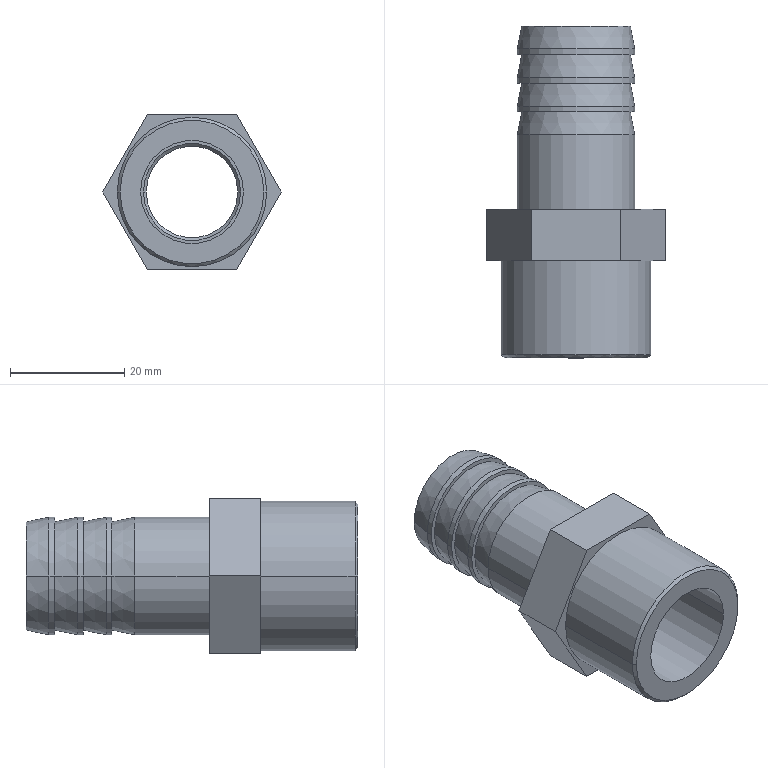Part | SolidWorks | features ICE 4, Chamfer 2, Revolution 1 | 1 solid | 40 faces | box 31.177 x 58 x 27 mm | volume 12376 mm3 | cylinder 14 | plane 14 | cone 12 | commonest cylinder face diameters 20.5 x8 16 x2 18 x2 26.1 x2
STEP:
#1=CARTESIAN_POINT('',(-8.,-8.5,0.));
#2=VERTEX_POINT('',#1);
#3=CARTESIAN_POINT('',(8.,-8.5,0.));
#4=VERTEX_POINT('',#3);
#5=CARTESIAN_POINT('',(0.,-8.5,0.));
#6=DIRECTION('',(0.,-1.,0.));
#7=DIRECTION('',(1.,0.,0.));
#8=AXIS2_PLACEMENT_3D('',#5,#6,#7);
#9=CIRCLE('',#8,8.);
#10=EDGE_CURVE('',#2,#4,#9,.T.);
#11=ORIENTED_EDGE('',*,*,#10,.F.);
#12=CARTESIAN_POINT('',(-8.5,-9.,0.));
#13=VERTEX_POINT('',#12);
#14=CARTESIAN_POINT('',(-8.5,-9.,0.));
#15=DIRECTION('',(-0.7071,-0.7071,0.));
#16=VECTOR('',#15,1000.);
#17=LINE('',#14,#16);
#18=EDGE_CURVE('',#2,#13,#17,.T.);
#19=ORIENTED_EDGE('',*,*,#18,.T.);
#20=CARTESIAN_POINT('',(8.5,-9.,0.));
#21=VERTEX_POINT('',#20);
#22=CARTESIAN_POINT('',(0.,-9.,0.));
#23=DIRECTION('',(0.,1.,0.));
#24=DIRECTION('',(1.,0.,0.));
#25=AXIS2_PLACEMENT_3D('',#22,#23,#24);
#26=CIRCLE('',#25,8.5);
#27=EDGE_CURVE('',#21,#13,#26,.T.);
#28=ORIENTED_EDGE('',*,*,#27,.F.);
#29=CARTESIAN_POINT('',(8.5,-9.,0.));
#30=DIRECTION('',(0.7071,-0.7071,0.));
#31=VECTOR('',#30,1000.);
#32=LINE('',#29,#31);
#33=EDGE_CURVE('',#4,#21,#32,.T.);
#34=ORIENTED_EDGE('',*,*,#33,.F.);
#35=EDGE_LOOP('',(#11,#19,#28,#34));
#36=FACE_OUTER_BOUND('',#35,.T.);
#37=CARTESIAN_POINT('',(0.,-9.,0.));
#38=DIRECTION('',(0.,-1.,0.));
#39=DIRECTION('',(1.,0.,0.));
#40=AXIS2_PLACEMENT_3D('',#37,#38,#39);
#41=CONICAL_SURFACE('',#40,8.5,0.7854);
#42=ADVANCED_FACE('',(#36),#41,.F.);
#43=CARTESIAN_POINT('',(12.55,-26.,0.));
#44=VERTEX_POINT('',#43);
#45=CARTESIAN_POINT('',(-12.55,-26.,0.));
#46=VERTEX_POINT('',#45);
#47=CARTESIAN_POINT('',(0.,-26.,0.));
#48=DIRECTION('',(0.,-1.,0.));
#49=DIRECTION('',(1.,0.,0.));
#50=AXIS2_PLACEMENT_3D('',#47,#48,#49);
#51=CIRCLE('',#50,12.55);
#52=EDGE_CURVE('',#44,#46,#51,.T.);
#53=ORIENTED_EDGE('',*,*,#52,.F.);
#54=CARTESIAN_POINT('',(13.05,-25.5,0.));
#55=VERTEX_POINT('',#54);
#56=CARTESIAN_POINT('',(12.55,-26.,0.));
#57=DIRECTION('',(0.7071,0.7071,0.));
#58=VECTOR('',#57,1000.);
#59=LINE('',#56,#58);
#60=EDGE_CURVE('',#44,#55,#59,.T.);
#61=ORIENTED_EDGE('',*,*,#60,.T.);
#62=CARTESIAN_POINT('',(-13.05,-25.5,0.));
#63=VERTEX_POINT('',#62);
#64=CARTESIAN_POINT('',(0.,-25.5,0.));
#65=DIRECTION('',(0.,1.,0.));
#66=DIRECTION('',(1.,0.,0.));
#67=AXIS2_PLACEMENT_3D('',#64,#65,#66);
#68=CIRCLE('',#67,13.05);
#69=EDGE_CURVE('',#63,#55,#68,.T.);
#70=ORIENTED_EDGE('',*,*,#69,.F.);
#71=CARTESIAN_POINT('',(-12.55,-26.,0.));
#72=DIRECTION('',(-0.7071,0.7071,0.));
#73=VECTOR('',#72,1000.);
#74=LINE('',#71,#73);
#75=EDGE_CURVE('',#46,#63,#74,.T.);
#76=ORIENTED_EDGE('',*,*,#75,.F.);
#77=EDGE_LOOP('',(#53,#61,#70,#76));
#78=FACE_OUTER_BOUND('',#77,.T.);
#79=CARTESIAN_POINT('',(0.,-26.,0.));
#80=DIRECTION('',(0.,1.,0.));
#81=DIRECTION('',(-1.,0.,0.));
#82=AXIS2_PLACEMENT_3D('',#79,#80,#81);
#83=CONICAL_SURFACE('',#82,12.55,0.7854);
#84=ADVANCED_FACE('',(#78),#83,.T.);
#85=CARTESIAN_POINT('',(9.,-9.,0.));
#86=VERTEX_POINT('',#85);
#87=CARTESIAN_POINT('',(-9.,-9.,0.));
#88=VERTEX_POINT('',#87);
#89=CARTESIAN_POINT('',(0.,-9.,0.));
#90=DIRECTION('',(0.,1.,0.));
#91=DIRECTION('',(1.,0.,0.));
#92=AXIS2_PLACEMENT_3D('',#89,#90,#91);
#93=CIRCLE('',#92,9.);
#94=EDGE_CURVE('',#86,#88,#93,.T.);
#95=ORIENTED_EDGE('',*,*,#94,.T.);
#96=CARTESIAN_POINT('',(-9.,-26.,0.));
#97=VERTEX_POINT('',#96);
#98=CARTESIAN_POINT('',(-9.,16.456,0.));
#99=DIRECTION('',(0.,-1.,0.));
#100=VECTOR('',#99,1000.);
#101=LINE('',#98,#100);
#102=EDGE_CURVE('',#88,#97,#101,.T.);
#103=ORIENTED_EDGE('',*,*,#102,.T.);
#104=CARTESIAN_POINT('',(9.,-26.,0.));
#105=VERTEX_POINT('',#104);
#106=CARTESIAN_POINT('',(0.,-26.,0.));
#107=DIRECTION('',(0.,-1.,0.));
#108=DIRECTION('',(1.,0.,0.));
#109=AXIS2_PLACEMENT_3D('',#106,#107,#108);
#110=CIRCLE('',#109,9.);
#111=EDGE_CURVE('',#97,#105,#110,.T.);
#112=ORIENTED_EDGE('',*,*,#111,.T.);
#113=CARTESIAN_POINT('',(9.,16.456,0.));
#114=DIRECTION('',(0.,-1.,0.));
#115=VECTOR('',#114,1000.);
#116=LINE('',#113,#115);
#117=EDGE_CURVE('',#86,#105,#116,.T.);
#118=ORIENTED_EDGE('',*,*,#117,.F.);
#119=EDGE_LOOP('',(#95,#103,#112,#118));
#120=FACE_OUTER_BOUND('',#119,.T.);
#121=CARTESIAN_POINT('',(0.,16.456,0.));
#122=DIRECTION('',(0.,-1.,0.));
#123=DIRECTION('',(1.,0.,0.));
#124=AXIS2_PLACEMENT_3D('',#121,#122,#123);
#125=CYLINDRICAL_SURFACE('',#124,9.);
#126=ADVANCED_FACE('',(#120),#125,.F.);
#127=ORIENTED_EDGE('',*,*,#69,.T.);
#128=CARTESIAN_POINT('',(13.05,-9.,0.));
#129=VERTEX_POINT('',#128);
#130=CARTESIAN_POINT('',(13.05,-26.,0.));
#131=DIRECTION('',(0.,1.,0.));
#132=VECTOR('',#131,1000.);
#133=LINE('',#130,#132);
#134=EDGE_CURVE('',#55,#129,#133,.T.);
#135=ORIENTED_EDGE('',*,*,#134,.T.);
#136=CARTESIAN_POINT('',(-13.05,-9.,0.));
#137=VERTEX_POINT('',#136);
#138=CARTESIAN_POINT('',(0.,-9.,0.));
#139=DIRECTION('',(0.,-1.,0.));
#140=DIRECTION('',(1.,0.,0.));
#141=AXIS2_PLACEMENT_3D('',#138,#139,#140);
#142=CIRCLE('',#141,13.05);
#143=EDGE_CURVE('',#129,#137,#142,.T.);
#144=ORIENTED_EDGE('',*,*,#143,.T.);
#145=CARTESIAN_POINT('',(-13.05,-26.,0.));
#146=DIRECTION('',(0.,1.,0.));
#147=VECTOR('',#146,1000.);
#148=LINE('',#145,#147);
#149=EDGE_CURVE('',#63,#137,#148,.T.);
#150=ORIENTED_EDGE('',*,*,#149,.F.);
#151=EDGE_LOOP('',(#127,#135,#144,#150));
#152=FACE_OUTER_BOUND('',#151,.T.);
#153=CARTESIAN_POINT('',(0.,-26.,0.));
#154=DIRECTION('',(0.,1.,0.));
#155=DIRECTION('',(-1.,0.,0.));
#156=AXIS2_PLACEMENT_3D('',#153,#154,#155);
#157=CYLINDRICAL_SURFACE('',#156,13.05);
#158=ADVANCED_FACE('',(#152),#157,.T.);
#159=CARTESIAN_POINT('',(9.5,32.,0.));
#160=VERTEX_POINT('',#159);
#161=CARTESIAN_POINT('',(-9.5,32.,0.));
#162=VERTEX_POINT('',#161);
#163=CARTESIAN_POINT('',(0.,32.,0.));
#164=DIRECTION('',(0.,-1.,0.));
#165=DIRECTION('',(1.,0.,0.));
#166=AXIS2_PLACEMENT_3D('',#163,#164,#165);
#167=CIRCLE('',#166,9.5);
#168=EDGE_CURVE('',#160,#162,#167,.T.);
#169=ORIENTED_EDGE('',*,*,#168,.T.);
#170=CARTESIAN_POINT('',(-10.25,28.,0.));
#171=VERTEX_POINT('',#170);
#172=CARTESIAN_POINT('',(-9.5,32.,0.));
#173=DIRECTION('',(-0.1843,-0.9829,0.));
#174=VECTOR('',#173,1000.);
#175=LINE('',#172,#174);
#176=EDGE_CURVE('',#162,#171,#175,.T.);
#177=ORIENTED_EDGE('',*,*,#176,.T.);
#178=CARTESIAN_POINT('',(10.25,28.,0.));
#179=VERTEX_POINT('',#178);
#180=CARTESIAN_POINT('',(0.,28.,0.));
#181=DIRECTION('',(0.,-1.,0.));
#182=DIRECTION('',(1.,0.,0.));
#183=AXIS2_PLACEMENT_3D('',#180,#181,#182);
#184=CIRCLE('',#183,10.25);
#185=EDGE_CURVE('',#179,#171,#184,.T.);
#186=ORIENTED_EDGE('',*,*,#185,.F.);
#187=CARTESIAN_POINT('',(9.5,32.,0.));
#188=DIRECTION('',(0.1843,-0.9829,0.));
#189=VECTOR('',#188,1000.);
#190=LINE('',#187,#189);
#191=EDGE_CURVE('',#160,#179,#190,.T.);
#192=ORIENTED_EDGE('',*,*,#191,.F.);
#193=EDGE_LOOP('',(#169,#177,#186,#192));
#194=FACE_OUTER_BOUND('',#193,.T.);
#195=CARTESIAN_POINT('',(0.,32.,0.));
#196=DIRECTION('',(0.,-1.,0.));
#197=DIRECTION('',(1.,0.,0.));
#198=AXIS2_PLACEMENT_3D('',#195,#196,#197);
#199=CONICAL_SURFACE('',#198,9.5,0.1853);
#200=ADVANCED_FACE('',(#194),#199,.T.);
#201=ORIENTED_EDGE('',*,*,#185,.T.);
#202=CARTESIAN_POINT('',(-10.25,27.,0.));
#203=VERTEX_POINT('',#202);
#204=CARTESIAN_POINT('',(-10.25,0.,0.));
#205=DIRECTION('',(0.,-1.,0.));
#206=VECTOR('',#205,1000.);
#207=LINE('',#204,#206);
#208=EDGE_CURVE('',#171,#203,#207,.T.);
#209=ORIENTED_EDGE('',*,*,#208,.T.);
#210=CARTESIAN_POINT('',(10.25,27.,0.));
#211=VERTEX_POINT('',#210);
#212=CARTESIAN_POINT('',(0.,27.,0.));
#213=DIRECTION('',(0.,-1.,0.));
#214=DIRECTION('',(1.,0.,0.));
#215=AXIS2_PLACEMENT_3D('',#212,#213,#214);
#216=CIRCLE('',#215,10.25);
#217=EDGE_CURVE('',#211,#203,#216,.T.);
#218=ORIENTED_EDGE('',*,*,#217,.F.);
#219=CARTESIAN_POINT('',(10.25,0.,0.));
#220=DIRECTION('',(0.,-1.,0.));
#221=VECTOR('',#220,1000.);
#222=LINE('',#219,#221);
#223=EDGE_CURVE('',#179,#211,#222,.T.);
#224=ORIENTED_EDGE('',*,*,#223,.F.);
#225=EDGE_LOOP('',(#201,#209,#218,#224));
#226=FACE_OUTER_BOUND('',#225,.T.);
#227=CARTESIAN_POINT('',(0.,0.,0.));
#228=DIRECTION('',(0.,-1.,0.));
#229=DIRECTION('',(1.,0.,0.));
#230=AXIS2_PLACEMENT_3D('',#227,#228,#229);
#231=CYLINDRICAL_SURFACE('',#230,10.25);
#232=ADVANCED_FACE('',(#226),#231,.T.);
#233=CARTESIAN_POINT('',(9.5,27.,0.));
#234=VERTEX_POINT('',#233);
#235=CARTESIAN_POINT('',(-9.5,27.,0.));
#236=VERTEX_POINT('',#235);
#237=CARTESIAN_POINT('',(0.,27.,0.));
#238=DIRECTION('',(0.,-1.,0.));
#239=DIRECTION('',(1.,0.,0.));
#240=AXIS2_PLACEMENT_3D('',#237,#238,#239);
#241=CIRCLE('',#240,9.5);
#242=EDGE_CURVE('',#234,#236,#241,.T.);
#243=ORIENTED_EDGE('',*,*,#242,.T.);
#244=CARTESIAN_POINT('',(-10.25,23.,0.));
#245=VERTEX_POINT('',#244);
#246=CARTESIAN_POINT('',(-9.5,27.,0.));
#247=DIRECTION('',(-0.1843,-0.9829,0.));
#248=VECTOR('',#247,1000.);
#249=LINE('',#246,#248);
#250=EDGE_CURVE('',#236,#245,#249,.T.);
#251=ORIENTED_EDGE('',*,*,#250,.T.);
#252=CARTESIAN_POINT('',(10.25,23.,0.));
#253=VERTEX_POINT('',#252);
#254=CARTESIAN_POINT('',(0.,23.,0.));
#255=DIRECTION('',(0.,-1.,0.));
#256=DIRECTION('',(1.,0.,0.));
#257=AXIS2_PLACEMENT_3D('',#254,#255,#256);
#258=CIRCLE('',#257,10.25);
#259=EDGE_CURVE('',#253,#245,#258,.T.);
#260=ORIENTED_EDGE('',*,*,#259,.F.);
#261=CARTESIAN_POINT('',(9.5,27.,0.));
#262=DIRECTION('',(0.1843,-0.9829,0.));
#263=VECTOR('',#262,1000.);
#264=LINE('',#261,#263);
#265=EDGE_CURVE('',#234,#253,#264,.T.);
#266=ORIENTED_EDGE('',*,*,#265,.F.);
#267=EDGE_LOOP('',(#243,#251,#260,#266));
#268=FACE_OUTER_BOUND('',#267,.T.);
#269=CARTESIAN_POINT('',(0.,27.,0.));
#270=DIRECTION('',(0.,-1.,0.));
#271=DIRECTION('',(1.,0.,0.));
#272=AXIS2_PLACEMENT_3D('',#269,#270,#271);
#273=CONICAL_SURFACE('',#272,9.5,0.1853);
#274=ADVANCED_FACE('',(#268),#273,.T.);
#275=ORIENTED_EDGE('',*,*,#259,.T.);
#276=CARTESIAN_POINT('',(-10.25,22.,0.));
#277=VERTEX_POINT('',#276);
#278=CARTESIAN_POINT('',(-10.25,0.,0.));
#279=DIRECTION('',(0.,-1.,0.));
#280=VECTOR('',#279,1000.);
#281=LINE('',#278,#280);
#282=EDGE_CURVE('',#245,#277,#281,.T.);
#283=ORIENTED_EDGE('',*,*,#282,.T.);
#284=CARTESIAN_POINT('',(10.25,22.,0.));
#285=VERTEX_POINT('',#284);
#286=CARTESIAN_POINT('',(0.,22.,0.));
#287=DIRECTION('',(0.,-1.,0.));
#288=DIRECTION('',(1.,0.,0.));
#289=AXIS2_PLACEMENT_3D('',#286,#287,#288);
#290=CIRCLE('',#289,10.25);
#291=EDGE_CURVE('',#285,#277,#290,.T.);
#292=ORIENTED_EDGE('',*,*,#291,.F.);
#293=CARTESIAN_POINT('',(10.25,0.,0.));
#294=DIRECTION('',(0.,-1.,0.));
#295=VECTOR('',#294,1000.);
#296=LINE('',#293,#295);
#297=EDGE_CURVE('',#253,#285,#296,.T.);
#298=ORIENTED_EDGE('',*,*,#297,.F.);
#299=EDGE_LOOP('',(#275,#283,#292,#298));
#300=FACE_OUTER_BOUND('',#299,.T.);
#301=CARTESIAN_POINT('',(0.,0.,0.));
#302=DIRECTION('',(0.,-1.,0.));
#303=DIRECTION('',(1.,0.,0.));
#304=AXIS2_PLACEMENT_3D('',#301,#302,#303);
#305=CYLINDRICAL_SURFACE('',#304,10.25);
#306=ADVANCED_FACE('',(#300),#305,.T.);
#307=CARTESIAN_POINT('',(9.5,22.,0.));
#308=VERTEX_POINT('',#307);
#309=CARTESIAN_POINT('',(-9.5,22.,0.));
#310=VERTEX_POINT('',#309);
#311=CARTESIAN_POINT('',(0.,22.,0.));
#312=DIRECTION('',(0.,-1.,0.));
#313=DIRECTION('',(1.,0.,0.));
#314=AXIS2_PLACEMENT_3D('',#311,#312,#313);
#315=CIRCLE('',#314,9.5);
#316=EDGE_CURVE('',#308,#310,#315,.T.);
#317=ORIENTED_EDGE('',*,*,#316,.T.);
#318=CARTESIAN_POINT('',(-10.25,18.,0.));
#319=VERTEX_POINT('',#318);
#320=CARTESIAN_POINT('',(-9.5,22.,0.));
#321=DIRECTION('',(-0.1843,-0.9829,0.));
#322=VECTOR('',#321,1000.);
#323=LINE('',#320,#322);
#324=EDGE_CURVE('',#310,#319,#323,.T.);
#325=ORIENTED_EDGE('',*,*,#324,.T.);
#326=CARTESIAN_POINT('',(10.25,18.,0.));
#327=VERTEX_POINT('',#326);
#328=CARTESIAN_POINT('',(0.,18.,0.));
#329=DIRECTION('',(0.,-1.,0.));
#330=DIRECTION('',(1.,0.,0.));
#331=AXIS2_PLACEMENT_3D('',#328,#329,#330);
#332=CIRCLE('',#331,10.25);
#333=EDGE_CURVE('',#327,#319,#332,.T.);
#334=ORIENTED_EDGE('',*,*,#333,.F.);
#335=CARTESIAN_POINT('',(9.5,22.,0.));
#336=DIRECTION('',(0.1843,-0.9829,0.));
#337=VECTOR('',#336,1000.);
#338=LINE('',#335,#337);
#339=EDGE_CURVE('',#308,#327,#338,.T.);
#340=ORIENTED_EDGE('',*,*,#339,.F.);
#341=EDGE_LOOP('',(#317,#325,#334,#340));
#342=FACE_OUTER_BOUND('',#341,.T.);
#343=CARTESIAN_POINT('',(0.,22.,0.));
#344=DIRECTION('',(0.,-1.,0.));
#345=DIRECTION('',(1.,0.,0.));
#346=AXIS2_PLACEMENT_3D('',#343,#344,#345);
#347=CONICAL_SURFACE('',#346,9.5,0.1853);
#348=ADVANCED_FACE('',(#342),#347,.T.);
#349=ORIENTED_EDGE('',*,*,#333,.T.);
#350=CARTESIAN_POINT('',(-10.25,17.,0.));
#351=VERTEX_POINT('',#350);
#352=CARTESIAN_POINT('',(-10.25,0.,0.));
#353=DIRECTION('',(0.,-1.,0.));
#354=VECTOR('',#353,1000.);
#355=LINE('',#352,#354);
#356=EDGE_CURVE('',#319,#351,#355,.T.);
#357=ORIENTED_EDGE('',*,*,#356,.T.);
#358=CARTESIAN_POINT('',(10.25,17.,0.));
#359=VERTEX_POINT('',#358);
#360=CARTESIAN_POINT('',(0.,17.,0.));
#361=DIRECTION('',(0.,-1.,0.));
#362=DIRECTION('',(1.,0.,0.));
#363=AXIS2_PLACEMENT_3D('',#360,#361,#362);
#364=CIRCLE('',#363,10.25);
#365=EDGE_CURVE('',#359,#351,#364,.T.);
#366=ORIENTED_EDGE('',*,*,#365,.F.);
#367=CARTESIAN_POINT('',(10.25,0.,0.));
#368=DIRECTION('',(0.,-1.,0.));
#369=VECTOR('',#368,1000.);
#370=LINE('',#367,#369);
#371=EDGE_CURVE('',#327,#359,#370,.T.);
#372=ORIENTED_EDGE('',*,*,#371,.F.);
#373=EDGE_LOOP('',(#349,#357,#366,#372));
#374=FACE_OUTER_BOUND('',#373,.T.);
#375=CARTESIAN_POINT('',(0.,0.,0.));
#376=DIRECTION('',(0.,-1.,0.));
#377=DIRECTION('',(1.,0.,0.));
#378=AXIS2_PLACEMENT_3D('',#375,#376,#377);
#379=CYLINDRICAL_SURFACE('',#378,10.25);
#380=ADVANCED_FACE('',(#374),#379,.T.);
#381=CARTESIAN_POINT('',(9.5,17.,0.));
#382=VERTEX_POINT('',#381);
#383=CARTESIAN_POINT('',(-9.5,17.,0.));
#384=VERTEX_POINT('',#383);
#385=CARTESIAN_POINT('',(0.,17.,0.));
#386=DIRECTION('',(0.,-1.,0.));
#387=DIRECTION('',(1.,0.,0.));
#388=AXIS2_PLACEMENT_3D('',#385,#386,#387);
#389=CIRCLE('',#388,9.5);
#390=EDGE_CURVE('',#382,#384,#389,.T.);
#391=ORIENTED_EDGE('',*,*,#390,.T.);
#392=CARTESIAN_POINT('',(-10.25,13.,0.));
#393=VERTEX_POINT('',#392);
#394=CARTESIAN_POINT('',(-9.5,17.,0.));
#395=DIRECTION('',(-0.1843,-0.9829,0.));
#396=VECTOR('',#395,1000.);
#397=LINE('',#394,#396);
#398=EDGE_CURVE('',#384,#393,#397,.T.);
#399=ORIENTED_EDGE('',*,*,#398,.T.);
#400=CARTESIAN_POINT('',(10.25,13.,0.));
#401=VERTEX_POINT('',#400);
#402=CARTESIAN_POINT('',(0.,13.,0.));
#403=DIRECTION('',(0.,-1.,0.));
#404=DIRECTION('',(1.,0.,0.));
#405=AXIS2_PLACEMENT_3D('',#402,#403,#404);
#406=CIRCLE('',#405,10.25);
#407=EDGE_CURVE('',#401,#393,#406,.T.);
#408=ORIENTED_EDGE('',*,*,#407,.F.);
#409=CARTESIAN_POINT('',(9.5,17.,0.));
#410=DIRECTION('',(0.1843,-0.9829,0.));
#411=VECTOR('',#410,1000.);
#412=LINE('',#409,#411);
#413=EDGE_CURVE('',#382,#401,#412,.T.);
#414=ORIENTED_EDGE('',*,*,#413,.F.);
#415=EDGE_LOOP('',(#391,#399,#408,#414));
#416=FACE_OUTER_BOUND('',#415,.T.);
#417=CARTESIAN_POINT('',(0.,17.,0.));
#418=DIRECTION('',(0.,-1.,0.));
#419=DIRECTION('',(1.,0.,0.));
#420=AXIS2_PLACEMENT_3D('',#417,#418,#419);
#421=CONICAL_SURFACE('',#420,9.5,0.1853);
#422=ADVANCED_FACE('',(#416),#421,.T.);
#423=ORIENTED_EDGE('',*,*,#407,.T.);
#424=CARTESIAN_POINT('',(-10.25,0.,0.));
#425=VERTEX_POINT('',#424);
#426=CARTESIAN_POINT('',(-10.25,0.,0.));
#427=DIRECTION('',(0.,-1.,0.));
#428=VECTOR('',#427,1000.);
#429=LINE('',#426,#428);
#430=EDGE_CURVE('',#393,#425,#429,.T.);
#431=ORIENTED_EDGE('',*,*,#430,.T.);
#432=CARTESIAN_POINT('',(10.25,0.,0.));
#433=VERTEX_POINT('',#432);
#434=CARTESIAN_POINT('',(0.,0.,0.));
#435=DIRECTION('',(0.,-1.,0.));
#436=DIRECTION('',(1.,0.,0.));
#437=AXIS2_PLACEMENT_3D('',#434,#435,#436);
#438=CIRCLE('',#437,10.25);
#439=EDGE_CURVE('',#433,#425,#438,.T.);
#440=ORIENTED_EDGE('',*,*,#439,.F.);
#441=CARTESIAN_POINT('',(10.25,0.,0.));
#442=DIRECTION('',(0.,-1.,0.));
#443=VECTOR('',#442,1000.);
#444=LINE('',#441,#443);
#445=EDGE_CURVE('',#401,#433,#444,.T.);
#446=ORIENTED_EDGE('',*,*,#445,.F.);
#447=EDGE_LOOP('',(#423,#431,#440,#446));
#448=FACE_OUTER_BOUND('',#447,.T.);
#449=CARTESIAN_POINT('',(0.,0.,0.));
#450=DIRECTION('',(0.,-1.,0.));
#451=DIRECTION('',(1.,0.,0.));
#452=AXIS2_PLACEMENT_3D('',#449,#450,#451);
#453=CYLINDRICAL_SURFACE('',#452,10.25);
#454=ADVANCED_FACE('',(#448),#453,.T.);
#455=ORIENTED_EDGE('',*,*,#10,.T.);
#456=CARTESIAN_POINT('',(8.,32.,0.));
#457=VERTEX_POINT('',#456);
#458=CARTESIAN_POINT('',(8.,-26.001,0.));
#459=DIRECTION('',(0.,1.,0.));
#460=VECTOR('',#459,1000.);
#461=LINE('',#458,#460);
#462=EDGE_CURVE('',#4,#457,#461,.T.);
#463=ORIENTED_EDGE('',*,*,#462,.T.);
#464=CARTESIAN_POINT('',(-8.,32.,0.));
#465=VERTEX_POINT('',#464);
#466=CARTESIAN_POINT('',(0.,32.,0.));
#467=DIRECTION('',(0.,1.,0.));
#468=DIRECTION('',(-1.,0.,0.));
#469=AXIS2_PLACEMENT_3D('',#466,#467,#468);
#470=CIRCLE('',#469,8.);
#471=EDGE_CURVE('',#457,#465,#470,.T.);
#472=ORIENTED_EDGE('',*,*,#471,.T.);
#473=CARTESIAN_POINT('',(-8.,-26.001,0.));
#474=DIRECTION('',(0.,1.,0.));
#475=VECTOR('',#474,1000.);
#476=LINE('',#473,#475);
#477=EDGE_CURVE('',#2,#465,#476,.T.);
#478=ORIENTED_EDGE('',*,*,#477,.F.);
#479=EDGE_LOOP('',(#455,#463,#472,#478));
#480=FACE_OUTER_BOUND('',#479,.T.);
#481=CARTESIAN_POINT('',(0.,-26.001,0.));
#482=DIRECTION('',(0.,1.,0.));
#483=DIRECTION('',(-1.,0.,0.));
#484=AXIS2_PLACEMENT_3D('',#481,#482,#483);
#485=CYLINDRICAL_SURFACE('',#484,8.);
#486=ADVANCED_FACE('',(#480),#485,.F.);
#487=ORIENTED_EDGE('',*,*,#462,.F.);
#488=CARTESIAN_POINT('',(0.,-8.5,0.));
#489=DIRECTION('',(0.,-1.,0.));
#490=DIRECTION('',(1.,0.,0.));
#491=AXIS2_PLACEMENT_3D('',#488,#489,#490);
#492=CIRCLE('',#491,8.);
#493=EDGE_CURVE('',#4,#2,#492,.T.);
#494=ORIENTED_EDGE('',*,*,#493,.T.);
#495=ORIENTED_EDGE('',*,*,#477,.T.);
#496=CARTESIAN_POINT('',(0.,32.,0.));
#497=DIRECTION('',(0.,1.,0.));
#498=DIRECTION('',(-1.,0.,0.));
#499=AXIS2_PLACEMENT_3D('',#496,#497,#498);
#500=CIRCLE('',#499,8.);
#501=EDGE_CURVE('',#465,#457,#500,.T.);
#502=ORIENTED_EDGE('',*,*,#501,.T.);
#503=EDGE_LOOP('',(#487,#494,#495,#502));
#504=FACE_OUTER_BOUND('',#503,.T.);
#505=CARTESIAN_POINT('',(0.,-26.001,0.));
#506=DIRECTION('',(0.,1.,0.));
#507=DIRECTION('',(-1.,0.,0.));
#508=AXIS2_PLACEMENT_3D('',#505,#506,#507);
#509=CYLINDRICAL_SURFACE('',#508,8.);
#510=ADVANCED_FACE('',(#504),#509,.F.);
#511=ORIENTED_EDGE('',*,*,#430,.F.);
#512=CARTESIAN_POINT('',(0.,13.,0.));
#513=DIRECTION('',(0.,-1.,0.));
#514=DIRECTION('',(1.,0.,0.));
#515=AXIS2_PLACEMENT_3D('',#512,#513,#514);
#516=CIRCLE('',#515,10.25);
#517=EDGE_CURVE('',#393,#401,#516,.T.);
#518=ORIENTED_EDGE('',*,*,#517,.T.);
#519=ORIENTED_EDGE('',*,*,#445,.T.);
#520=CARTESIAN_POINT('',(0.,0.,0.));
#521=DIRECTION('',(0.,-1.,0.));
#522=DIRECTION('',(1.,0.,0.));
#523=AXIS2_PLACEMENT_3D('',#520,#521,#522);
#524=CIRCLE('',#523,10.25);
#525=EDGE_CURVE('',#425,#433,#524,.T.);
#526=ORIENTED_EDGE('',*,*,#525,.F.);
#527=EDGE_LOOP('',(#511,#518,#519,#526));
#528=FACE_OUTER_BOUND('',#527,.T.);
#529=CARTESIAN_POINT('',(0.,0.,0.));
#530=DIRECTION('',(0.,-1.,0.));
#531=DIRECTION('',(1.,0.,0.));
#532=AXIS2_PLACEMENT_3D('',#529,#530,#531);
#533=CYLINDRICAL_SURFACE('',#532,10.25);
#534=ADVANCED_FACE('',(#528),#533,.T.);
#535=ORIENTED_EDGE('',*,*,#398,.F.);
#536=CARTESIAN_POINT('',(0.,17.,0.));
#537=DIRECTION('',(0.,-1.,0.));
#538=DIRECTION('',(1.,0.,0.));
#539=AXIS2_PLACEMENT_3D('',#536,#537,#538);
#540=CIRCLE('',#539,9.5);
#541=EDGE_CURVE('',#384,#382,#540,.T.);
#542=ORIENTED_EDGE('',*,*,#541,.T.);
#543=ORIENTED_EDGE('',*,*,#413,.T.);
#544=ORIENTED_EDGE('',*,*,#517,.F.);
#545=EDGE_LOOP('',(#535,#542,#543,#544));
#546=FACE_OUTER_BOUND('',#545,.T.);
#547=CARTESIAN_POINT('',(0.,17.,0.));
#548=DIRECTION('',(0.,-1.,0.));
#549=DIRECTION('',(1.,0.,0.));
#550=AXIS2_PLACEMENT_3D('',#547,#548,#549);
#551=CONICAL_SURFACE('',#550,9.5,0.1853);
#552=ADVANCED_FACE('',(#546),#551,.T.);
#553=ORIENTED_EDGE('',*,*,#390,.F.);
#554=ORIENTED_EDGE('',*,*,#541,.F.);
#555=EDGE_LOOP('',(#553,#554));
#556=FACE_BOUND('',#555,.T.);
#557=ORIENTED_EDGE('',*,*,#365,.T.);
#558=CARTESIAN_POINT('',(0.,17.,0.));
#559=DIRECTION('',(0.,-1.,0.));
#560=DIRECTION('',(1.,0.,0.));
#561=AXIS2_PLACEMENT_3D('',#558,#559,#560);
#562=CIRCLE('',#561,10.25);
#563=EDGE_CURVE('',#351,#359,#562,.T.);
#564=ORIENTED_EDGE('',*,*,#563,.T.);
#565=EDGE_LOOP('',(#557,#564));
#566=FACE_OUTER_BOUND('',#565,.T.);
#567=CARTESIAN_POINT('',(-10.25,17.,0.));
#568=DIRECTION('',(0.,1.,0.));
#569=DIRECTION('',(-1.,0.,0.));
#570=AXIS2_PLACEMENT_3D('',#567,#568,#569);
#571=PLANE('',#570);
#572=ADVANCED_FACE('',(#556,#566),#571,.F.);
#573=ORIENTED_EDGE('',*,*,#356,.F.);
#574=CARTESIAN_POINT('',(0.,18.,0.));
#575=DIRECTION('',(0.,-1.,0.));
#576=DIRECTION('',(1.,0.,0.));
#577=AXIS2_PLACEMENT_3D('',#574,#575,#576);
#578=CIRCLE('',#577,10.25);
#579=EDGE_CURVE('',#319,#327,#578,.T.);
#580=ORIENTED_EDGE('',*,*,#579,.T.);
#581=ORIENTED_EDGE('',*,*,#371,.T.);
#582=ORIENTED_EDGE('',*,*,#563,.F.);
#583=EDGE_LOOP('',(#573,#580,#581,#582));
#584=FACE_OUTER_BOUND('',#583,.T.);
#585=CARTESIAN_POINT('',(0.,0.,0.));
#586=DIRECTION('',(0.,-1.,0.));
#587=DIRECTION('',(1.,0.,0.));
#588=AXIS2_PLACEMENT_3D('',#585,#586,#587);
#589=CYLINDRICAL_SURFACE('',#588,10.25);
#590=ADVANCED_FACE('',(#584),#589,.T.);
#591=ORIENTED_EDGE('',*,*,#324,.F.);
#592=CARTESIAN_POINT('',(0.,22.,0.));
#593=DIRECTION('',(0.,-1.,0.));
#594=DIRECTION('',(1.,0.,0.));
#595=AXIS2_PLACEMENT_3D('',#592,#593,#594);
#596=CIRCLE('',#595,9.5);
#597=EDGE_CURVE('',#310,#308,#596,.T.);
#598=ORIENTED_EDGE('',*,*,#597,.T.);
#599=ORIENTED_EDGE('',*,*,#339,.T.);
#600=ORIENTED_EDGE('',*,*,#579,.F.);
#601=EDGE_LOOP('',(#591,#598,#599,#600));
#602=FACE_OUTER_BOUND('',#601,.T.);
#603=CARTESIAN_POINT('',(0.,22.,0.));
#604=DIRECTION('',(0.,-1.,0.));
#605=DIRECTION('',(1.,0.,0.));
#606=AXIS2_PLACEMENT_3D('',#603,#604,#605);
#607=CONICAL_SURFACE('',#606,9.5,0.1853);
#608=ADVANCED_FACE('',(#602),#607,.T.);
#609=ORIENTED_EDGE('',*,*,#316,.F.);
#610=ORIENTED_EDGE('',*,*,#597,.F.);
#611=EDGE_LOOP('',(#609,#610));
#612=FACE_BOUND('',#611,.T.);
#613=ORIENTED_EDGE('',*,*,#291,.T.);
#614=CARTESIAN_POINT('',(0.,22.,0.));
#615=DIRECTION('',(0.,-1.,0.));
#616=DIRECTION('',(1.,0.,0.));
#617=AXIS2_PLACEMENT_3D('',#614,#615,#616);
#618=CIRCLE('',#617,10.25);
#619=EDGE_CURVE('',#277,#285,#618,.T.);
#620=ORIENTED_EDGE('',*,*,#619,.T.);
#621=EDGE_LOOP('',(#613,#620));
#622=FACE_OUTER_BOUND('',#621,.T.);
#623=CARTESIAN_POINT('',(-10.25,22.,0.));
#624=DIRECTION('',(0.,1.,0.));
#625=DIRECTION('',(-1.,0.,0.));
#626=AXIS2_PLACEMENT_3D('',#623,#624,#625);
#627=PLANE('',#626);
#628=ADVANCED_FACE('',(#612,#622),#627,.F.);
#629=ORIENTED_EDGE('',*,*,#282,.F.);
#630=CARTESIAN_POINT('',(0.,23.,0.));
#631=DIRECTION('',(0.,-1.,0.));
#632=DIRECTION('',(1.,0.,0.));
#633=AXIS2_PLACEMENT_3D('',#630,#631,#632);
#634=CIRCLE('',#633,10.25);
#635=EDGE_CURVE('',#245,#253,#634,.T.);
#636=ORIENTED_EDGE('',*,*,#635,.T.);
#637=ORIENTED_EDGE('',*,*,#297,.T.);
#638=ORIENTED_EDGE('',*,*,#619,.F.);
#639=EDGE_LOOP('',(#629,#636,#637,#638));
#640=FACE_OUTER_BOUND('',#639,.T.);
#641=CARTESIAN_POINT('',(0.,0.,0.));
#642=DIRECTION('',(0.,-1.,0.));
#643=DIRECTION('',(1.,0.,0.));
#644=AXIS2_PLACEMENT_3D('',#641,#642,#643);
#645=CYLINDRICAL_SURFACE('',#644,10.25);
#646=ADVANCED_FACE('',(#640),#645,.T.);
#647=ORIENTED_EDGE('',*,*,#250,.F.);
#648=CARTESIAN_POINT('',(0.,27.,0.));
#649=DIRECTION('',(0.,-1.,0.));
#650=DIRECTION('',(1.,0.,0.));
#651=AXIS2_PLACEMENT_3D('',#648,#649,#650);
#652=CIRCLE('',#651,9.5);
#653=EDGE_CURVE('',#236,#234,#652,.T.);
#654=ORIENTED_EDGE('',*,*,#653,.T.);
#655=ORIENTED_EDGE('',*,*,#265,.T.);
#656=ORIENTED_EDGE('',*,*,#635,.F.);
#657=EDGE_LOOP('',(#647,#654,#655,#656));
#658=FACE_OUTER_BOUND('',#657,.T.);
#659=CARTESIAN_POINT('',(0.,27.,0.));
#660=DIRECTION('',(0.,-1.,0.));
#661=DIRECTION('',(1.,0.,0.));
#662=AXIS2_PLACEMENT_3D('',#659,#660,#661);
#663=CONICAL_SURFACE('',#662,9.5,0.1853);
#664=ADVANCED_FACE('',(#658),#663,.T.);
#665=ORIENTED_EDGE('',*,*,#242,.F.);
#666=ORIENTED_EDGE('',*,*,#653,.F.);
#667=EDGE_LOOP('',(#665,#666));
#668=FACE_BOUND('',#667,.T.);
#669=ORIENTED_EDGE('',*,*,#217,.T.);
#670=CARTESIAN_POINT('',(0.,27.,0.));
#671=DIRECTION('',(0.,-1.,0.));
#672=DIRECTION('',(1.,0.,0.));
#673=AXIS2_PLACEMENT_3D('',#670,#671,#672);
#674=CIRCLE('',#673,10.25);
#675=EDGE_CURVE('',#203,#211,#674,.T.);
#676=ORIENTED_EDGE('',*,*,#675,.T.);
#677=EDGE_LOOP('',(#669,#676));
#678=FACE_OUTER_BOUND('',#677,.T.);
#679=CARTESIAN_POINT('',(-10.25,27.,0.));
#680=DIRECTION('',(0.,1.,0.));
#681=DIRECTION('',(-1.,0.,0.));
#682=AXIS2_PLACEMENT_3D('',#679,#680,#681);
#683=PLANE('',#682);
#684=ADVANCED_FACE('',(#668,#678),#683,.F.);
#685=ORIENTED_EDGE('',*,*,#208,.F.);
#686=CARTESIAN_POINT('',(0.,28.,0.));
#687=DIRECTION('',(0.,-1.,0.));
#688=DIRECTION('',(1.,0.,0.));
#689=AXIS2_PLACEMENT_3D('',#686,#687,#688);
#690=CIRCLE('',#689,10.25);
#691=EDGE_CURVE('',#171,#179,#690,.T.);
#692=ORIENTED_EDGE('',*,*,#691,.T.);
#693=ORIENTED_EDGE('',*,*,#223,.T.);
#694=ORIENTED_EDGE('',*,*,#675,.F.);
#695=EDGE_LOOP('',(#685,#692,#693,#694));
#696=FACE_OUTER_BOUND('',#695,.T.);
#697=CARTESIAN_POINT('',(0.,0.,0.));
#698=DIRECTION('',(0.,-1.,0.));
#699=DIRECTION('',(1.,0.,0.));
#700=AXIS2_PLACEMENT_3D('',#697,#698,#699);
#701=CYLINDRICAL_SURFACE('',#700,10.25);
#702=ADVANCED_FACE('',(#696),#701,.T.);
#703=ORIENTED_EDGE('',*,*,#176,.F.);
#704=CARTESIAN_POINT('',(0.,32.,0.));
#705=DIRECTION('',(0.,-1.,0.));
#706=DIRECTION('',(1.,0.,0.));
#707=AXIS2_PLACEMENT_3D('',#704,#705,#706);
#708=CIRCLE('',#707,9.5);
#709=EDGE_CURVE('',#162,#160,#708,.T.);
#710=ORIENTED_EDGE('',*,*,#709,.T.);
#711=ORIENTED_EDGE('',*,*,#191,.T.);
#712=ORIENTED_EDGE('',*,*,#691,.F.);
#713=EDGE_LOOP('',(#703,#710,#711,#712));
#714=FACE_OUTER_BOUND('',#713,.T.);
#715=CARTESIAN_POINT('',(0.,32.,0.));
#716=DIRECTION('',(0.,-1.,0.));
#717=DIRECTION('',(1.,0.,0.));
#718=AXIS2_PLACEMENT_3D('',#715,#716,#717);
#719=CONICAL_SURFACE('',#718,9.5,0.1853);
#720=ADVANCED_FACE('',(#714),#719,.T.);
#721=ORIENTED_EDGE('',*,*,#501,.F.);
#722=ORIENTED_EDGE('',*,*,#471,.F.);
#723=EDGE_LOOP('',(#721,#722));
#724=FACE_BOUND('',#723,.T.);
#725=ORIENTED_EDGE('',*,*,#168,.F.);
#726=ORIENTED_EDGE('',*,*,#709,.F.);
#727=EDGE_LOOP('',(#725,#726));
#728=FACE_OUTER_BOUND('',#727,.T.);
#729=CARTESIAN_POINT('',(-9.5,32.,0.));
#730=DIRECTION('',(0.,-1.,0.));
#731=DIRECTION('',(1.,0.,0.));
#732=AXIS2_PLACEMENT_3D('',#729,#730,#731);
#733=PLANE('',#732);
#734=ADVANCED_FACE('',(#724,#728),#733,.F.);
#735=CARTESIAN_POINT('',(7.794,0.,-13.5));
#736=VERTEX_POINT('',#735);
#737=CARTESIAN_POINT('',(15.588,0.,0.));
#738=VERTEX_POINT('',#737);
#739=CARTESIAN_POINT('',(7.794,0.,-13.5));
#740=DIRECTION('',(0.5,0.,0.866));
#741=VECTOR('',#740,1000.);
#742=LINE('',#739,#741);
#743=EDGE_CURVE('',#736,#738,#742,.T.);
#744=ORIENTED_EDGE('',*,*,#743,.T.);
#745=CARTESIAN_POINT('',(15.588,-9.,0.));
#746=VERTEX_POINT('',#745);
#747=CARTESIAN_POINT('',(15.588,-9.,0.));
#748=DIRECTION('',(0.,1.,0.));
#749=VECTOR('',#748,1000.);
#750=LINE('',#747,#749);
#751=EDGE_CURVE('',#746,#738,#750,.T.);
#752=ORIENTED_EDGE('',*,*,#751,.F.);
#753=CARTESIAN_POINT('',(7.794,-9.,-13.5));
#754=VERTEX_POINT('',#753);
#755=CARTESIAN_POINT('',(7.794,-9.,-13.5));
#756=DIRECTION('',(0.5,0.,0.866));
#757=VECTOR('',#756,1000.);
#758=LINE('',#755,#757);
#759=EDGE_CURVE('',#754,#746,#758,.T.);
#760=ORIENTED_EDGE('',*,*,#759,.F.);
#761=CARTESIAN_POINT('',(7.794,-9.,-13.5));
#762=DIRECTION('',(0.,1.,0.));
#763=VECTOR('',#762,1000.);
#764=LINE('',#761,#763);
#765=EDGE_CURVE('',#754,#736,#764,.T.);
#766=ORIENTED_EDGE('',*,*,#765,.T.);
#767=EDGE_LOOP('',(#744,#752,#760,#766));
#768=FACE_OUTER_BOUND('',#767,.T.);
#769=CARTESIAN_POINT('',(7.794,-9.,-13.5));
#770=DIRECTION('',(-0.866,0.,0.5));
#771=DIRECTION('',(0.5,0.,0.866));
#772=AXIS2_PLACEMENT_3D('',#769,#770,#771);
#773=PLANE('',#772);
#774=ADVANCED_FACE('',(#768),#773,.F.);
#775=CARTESIAN_POINT('',(7.794,0.,13.5));
#776=VERTEX_POINT('',#775);
#777=CARTESIAN_POINT('',(15.588,0.,0.));
#778=DIRECTION('',(-0.5,0.,0.866));
#779=VECTOR('',#778,1000.);
#780=LINE('',#777,#779);
#781=EDGE_CURVE('',#738,#776,#780,.T.);
#782=ORIENTED_EDGE('',*,*,#781,.T.);
#783=CARTESIAN_POINT('',(7.794,-9.,13.5));
#784=VERTEX_POINT('',#783);
#785=CARTESIAN_POINT('',(7.794,-9.,13.5));
#786=DIRECTION('',(0.,1.,0.));
#787=VECTOR('',#786,1000.);
#788=LINE('',#785,#787);
#789=EDGE_CURVE('',#784,#776,#788,.T.);
#790=ORIENTED_EDGE('',*,*,#789,.F.);
#791=CARTESIAN_POINT('',(15.588,-9.,0.));
#792=DIRECTION('',(-0.5,0.,0.866));
#793=VECTOR('',#792,1000.);
#794=LINE('',#791,#793);
#795=EDGE_CURVE('',#746,#784,#794,.T.);
#796=ORIENTED_EDGE('',*,*,#795,.F.);
#797=ORIENTED_EDGE('',*,*,#751,.T.);
#798=EDGE_LOOP('',(#782,#790,#796,#797));
#799=FACE_OUTER_BOUND('',#798,.T.);
#800=CARTESIAN_POINT('',(15.588,-9.,0.));
#801=DIRECTION('',(-0.866,0.,-0.5));
#802=DIRECTION('',(-0.5,0.,0.866));
#803=AXIS2_PLACEMENT_3D('',#800,#801,#802);
#804=PLANE('',#803);
#805=ADVANCED_FACE('',(#799),#804,.F.);
#806=CARTESIAN_POINT('',(-7.794,0.,13.5));
#807=VERTEX_POINT('',#806);
#808=CARTESIAN_POINT('',(7.794,0.,13.5));
#809=DIRECTION('',(-1.,0.,0.));
#810=VECTOR('',#809,1000.);
#811=LINE('',#808,#810);
#812=EDGE_CURVE('',#776,#807,#811,.T.);
#813=ORIENTED_EDGE('',*,*,#812,.T.);
#814=CARTESIAN_POINT('',(-7.794,-9.,13.5));
#815=VERTEX_POINT('',#814);
#816=CARTESIAN_POINT('',(-7.794,-9.,13.5));
#817=DIRECTION('',(0.,1.,0.));
#818=VECTOR('',#817,1000.);
#819=LINE('',#816,#818);
#820=EDGE_CURVE('',#815,#807,#819,.T.);
#821=ORIENTED_EDGE('',*,*,#820,.F.);
#822=CARTESIAN_POINT('',(7.794,-9.,13.5));
#823=DIRECTION('',(-1.,0.,0.));
#824=VECTOR('',#823,1000.);
#825=LINE('',#822,#824);
#826=EDGE_CURVE('',#784,#815,#825,.T.);
#827=ORIENTED_EDGE('',*,*,#826,.F.);
#828=ORIENTED_EDGE('',*,*,#789,.T.);
#829=EDGE_LOOP('',(#813,#821,#827,#828));
#830=FACE_OUTER_BOUND('',#829,.T.);
#831=CARTESIAN_POINT('',(7.794,-9.,13.5));
#832=DIRECTION('',(0.,0.,-1.));
#833=DIRECTION('',(-1.,0.,0.));
#834=AXIS2_PLACEMENT_3D('',#831,#832,#833);
#835=PLANE('',#834);
#836=ADVANCED_FACE('',(#830),#835,.F.);
#837=CARTESIAN_POINT('',(-15.588,0.,0.));
#838=VERTEX_POINT('',#837);
#839=CARTESIAN_POINT('',(-7.794,0.,13.5));
#840=DIRECTION('',(-0.5,0.,-0.866));
#841=VECTOR('',#840,1000.);
#842=LINE('',#839,#841);
#843=EDGE_CURVE('',#807,#838,#842,.T.);
#844=ORIENTED_EDGE('',*,*,#843,.T.);
#845=CARTESIAN_POINT('',(-15.588,-9.,0.));
#846=VERTEX_POINT('',#845);
#847=CARTESIAN_POINT('',(-15.588,-9.,0.));
#848=DIRECTION('',(0.,1.,0.));
#849=VECTOR('',#848,1000.);
#850=LINE('',#847,#849);
#851=EDGE_CURVE('',#846,#838,#850,.T.);
#852=ORIENTED_EDGE('',*,*,#851,.F.);
#853=CARTESIAN_POINT('',(-7.794,-9.,13.5));
#854=DIRECTION('',(-0.5,0.,-0.866));
#855=VECTOR('',#854,1000.);
#856=LINE('',#853,#855);
#857=EDGE_CURVE('',#815,#846,#856,.T.);
#858=ORIENTED_EDGE('',*,*,#857,.F.);
#859=ORIENTED_EDGE('',*,*,#820,.T.);
#860=EDGE_LOOP('',(#844,#852,#858,#859));
#861=FACE_OUTER_BOUND('',#860,.T.);
#862=CARTESIAN_POINT('',(-7.794,-9.,13.5));
#863=DIRECTION('',(0.866,0.,-0.5));
#864=DIRECTION('',(-0.5,0.,-0.866));
#865=AXIS2_PLACEMENT_3D('',#862,#863,#864);
#866=PLANE('',#865);
#867=ADVANCED_FACE('',(#861),#866,.F.);
#868=CARTESIAN_POINT('',(-7.794,0.,-13.5));
#869=VERTEX_POINT('',#868);
#870=CARTESIAN_POINT('',(-15.588,0.,0.));
#871=DIRECTION('',(0.5,0.,-0.866));
#872=VECTOR('',#871,1000.);
#873=LINE('',#870,#872);
#874=EDGE_CURVE('',#838,#869,#873,.T.);
#875=ORIENTED_EDGE('',*,*,#874,.T.);
#876=CARTESIAN_POINT('',(-7.794,-9.,-13.5));
#877=VERTEX_POINT('',#876);
#878=CARTESIAN_POINT('',(-7.794,-9.,-13.5));
#879=DIRECTION('',(0.,1.,0.));
#880=VECTOR('',#879,1000.);
#881=LINE('',#878,#880);
#882=EDGE_CURVE('',#877,#869,#881,.T.);
#883=ORIENTED_EDGE('',*,*,#882,.F.);
#884=CARTESIAN_POINT('',(-15.588,-9.,0.));
#885=DIRECTION('',(0.5,0.,-0.866));
#886=VECTOR('',#885,1000.);
#887=LINE('',#884,#886);
#888=EDGE_CURVE('',#846,#877,#887,.T.);
#889=ORIENTED_EDGE('',*,*,#888,.F.);
#890=ORIENTED_EDGE('',*,*,#851,.T.);
#891=EDGE_LOOP('',(#875,#883,#889,#890));
#892=FACE_OUTER_BOUND('',#891,.T.);
#893=CARTESIAN_POINT('',(-15.588,-9.,0.));
#894=DIRECTION('',(0.866,0.,0.5));
#895=DIRECTION('',(0.5,0.,-0.866));
#896=AXIS2_PLACEMENT_3D('',#893,#894,#895);
#897=PLANE('',#896);
#898=ADVANCED_FACE('',(#892),#897,.F.);
#899=CARTESIAN_POINT('',(-7.794,0.,-13.5));
#900=DIRECTION('',(1.,0.,0.));
#901=VECTOR('',#900,1000.);
#902=LINE('',#899,#901);
#903=EDGE_CURVE('',#869,#736,#902,.T.);
#904=ORIENTED_EDGE('',*,*,#903,.T.);
#905=ORIENTED_EDGE('',*,*,#765,.F.);
#906=CARTESIAN_POINT('',(-7.794,-9.,-13.5));
#907=DIRECTION('',(1.,0.,0.));
#908=VECTOR('',#907,1000.);
#909=LINE('',#906,#908);
#910=EDGE_CURVE('',#877,#754,#909,.T.);
#911=ORIENTED_EDGE('',*,*,#910,.F.);
#912=ORIENTED_EDGE('',*,*,#882,.T.);
#913=EDGE_LOOP('',(#904,#905,#911,#912));
#914=FACE_OUTER_BOUND('',#913,.T.);
#915=CARTESIAN_POINT('',(-7.794,-9.,-13.5));
#916=DIRECTION('',(0.,0.,1.));
#917=DIRECTION('',(1.,0.,0.));
#918=AXIS2_PLACEMENT_3D('',#915,#916,#917);
#919=PLANE('',#918);
#920=ADVANCED_FACE('',(#914),#919,.F.);
#921=CARTESIAN_POINT('',(0.,-9.,0.));
#922=DIRECTION('',(0.,-1.,0.));
#923=DIRECTION('',(1.,0.,0.));
#924=AXIS2_PLACEMENT_3D('',#921,#922,#923);
#925=CIRCLE('',#924,13.05);
#926=EDGE_CURVE('',#137,#129,#925,.T.);
#927=ORIENTED_EDGE('',*,*,#926,.F.);
#928=ORIENTED_EDGE('',*,*,#143,.F.);
#929=EDGE_LOOP('',(#927,#928));
#930=FACE_BOUND('',#929,.T.);
#931=ORIENTED_EDGE('',*,*,#759,.T.);
#932=ORIENTED_EDGE('',*,*,#795,.T.);
#933=ORIENTED_EDGE('',*,*,#826,.T.);
#934=ORIENTED_EDGE('',*,*,#857,.T.);
#935=ORIENTED_EDGE('',*,*,#888,.T.);
#936=ORIENTED_EDGE('',*,*,#910,.T.);
#937=EDGE_LOOP('',(#931,#932,#933,#934,#935,#936));
#938=FACE_OUTER_BOUND('',#937,.T.);
#939=CARTESIAN_POINT('',(0.,-9.,0.));
#940=DIRECTION('',(0.,-1.,0.));
#941=DIRECTION('',(1.,0.,0.));
#942=AXIS2_PLACEMENT_3D('',#939,#940,#941);
#943=PLANE('',#942);
#944=ADVANCED_FACE('',(#930,#938),#943,.T.);
#945=ORIENTED_EDGE('',*,*,#439,.T.);
#946=ORIENTED_EDGE('',*,*,#525,.T.);
#947=EDGE_LOOP('',(#945,#946));
#948=FACE_BOUND('',#947,.T.);
#949=ORIENTED_EDGE('',*,*,#743,.F.);
#950=ORIENTED_EDGE('',*,*,#903,.F.);
#951=ORIENTED_EDGE('',*,*,#874,.F.);
#952=ORIENTED_EDGE('',*,*,#843,.F.);
#953=ORIENTED_EDGE('',*,*,#812,.F.);
#954=ORIENTED_EDGE('',*,*,#781,.F.);
#955=EDGE_LOOP('',(#949,#950,#951,#952,#953,#954));
#956=FACE_OUTER_BOUND('',#955,.T.);
#957=CARTESIAN_POINT('',(0.,0.,0.));
#958=DIRECTION('',(0.,-1.,0.));
#959=DIRECTION('',(1.,0.,0.));
#960=AXIS2_PLACEMENT_3D('',#957,#958,#959);
#961=PLANE('',#960);
#962=ADVANCED_FACE('',(#948,#956),#961,.F.);
#963=ORIENTED_EDGE('',*,*,#134,.F.);
#964=CARTESIAN_POINT('',(0.,-25.5,0.));
#965=DIRECTION('',(0.,1.,0.));
#966=DIRECTION('',(1.,0.,0.));
#967=AXIS2_PLACEMENT_3D('',#964,#965,#966);
#968=CIRCLE('',#967,13.05);
#969=EDGE_CURVE('',#55,#63,#968,.T.);
#970=ORIENTED_EDGE('',*,*,#969,.T.);
#971=ORIENTED_EDGE('',*,*,#149,.T.);
#972=ORIENTED_EDGE('',*,*,#926,.T.);
#973=EDGE_LOOP('',(#963,#970,#971,#972));
#974=FACE_OUTER_BOUND('',#973,.T.);
#975=CARTESIAN_POINT('',(0.,-26.,0.));
#976=DIRECTION('',(0.,1.,0.));
#977=DIRECTION('',(-1.,0.,0.));
#978=AXIS2_PLACEMENT_3D('',#975,#976,#977);
#979=CYLINDRICAL_SURFACE('',#978,13.05);
#980=ADVANCED_FACE('',(#974),#979,.T.);
#981=CARTESIAN_POINT('',(0.,-26.,0.));
#982=DIRECTION('',(0.,-1.,0.));
#983=DIRECTION('',(1.,0.,0.));
#984=AXIS2_PLACEMENT_3D('',#981,#982,#983);
#985=CIRCLE('',#984,12.55);
#986=EDGE_CURVE('',#46,#44,#985,.T.);
#987=ORIENTED_EDGE('',*,*,#986,.T.);
#988=ORIENTED_EDGE('',*,*,#52,.T.);
#989=EDGE_LOOP('',(#987,#988));
#990=FACE_OUTER_BOUND('',#989,.T.);
#991=CARTESIAN_POINT('',(0.,-26.,0.));
#992=DIRECTION('',(0.,-1.,0.));
#993=DIRECTION('',(1.,0.,0.));
#994=AXIS2_PLACEMENT_3D('',#991,#992,#993);
#995=CIRCLE('',#994,9.);
#996=EDGE_CURVE('',#105,#97,#995,.T.);
#997=ORIENTED_EDGE('',*,*,#996,.F.);
#998=ORIENTED_EDGE('',*,*,#111,.F.);
#999=EDGE_LOOP('',(#997,#998));
#1000=FACE_BOUND('',#999,.T.);
#1001=CARTESIAN_POINT('',(0.,-26.,0.));
#1002=DIRECTION('',(0.,-1.,0.));
#1003=DIRECTION('',(1.,0.,0.));
#1004=AXIS2_PLACEMENT_3D('',#1001,#1002,#1003);
#1005=PLANE('',#1004);
#1006=ADVANCED_FACE('',(#990,#1000),#1005,.T.);
#1007=ORIENTED_EDGE('',*,*,#27,.T.);
#1008=CARTESIAN_POINT('',(0.,-9.,0.));
#1009=DIRECTION('',(0.,1.,0.));
#1010=DIRECTION('',(1.,0.,0.));
#1011=AXIS2_PLACEMENT_3D('',#1008,#1009,#1010);
#1012=CIRCLE('',#1011,8.5);
#1013=EDGE_CURVE('',#13,#21,#1012,.T.);
#1014=ORIENTED_EDGE('',*,*,#1013,.T.);
#1015=EDGE_LOOP('',(#1007,#1014));
#1016=FACE_BOUND('',#1015,.T.);
#1017=ORIENTED_EDGE('',*,*,#94,.F.);
#1018=CARTESIAN_POINT('',(0.,-9.,0.));
#1019=DIRECTION('',(0.,1.,0.));
#1020=DIRECTION('',(1.,0.,0.));
#1021=AXIS2_PLACEMENT_3D('',#1018,#1019,#1020);
#1022=CIRCLE('',#1021,9.);
#1023=EDGE_CURVE('',#88,#86,#1022,.T.);
#1024=ORIENTED_EDGE('',*,*,#1023,.F.);
#1025=EDGE_LOOP('',(#1017,#1024));
#1026=FACE_OUTER_BOUND('',#1025,.T.);
#1027=CARTESIAN_POINT('',(0.,-9.,0.));
#1028=DIRECTION('',(0.,-1.,0.));
#1029=DIRECTION('',(1.,0.,0.));
#1030=AXIS2_PLACEMENT_3D('',#1027,#1028,#1029);
#1031=PLANE('',#1030);
#1032=ADVANCED_FACE('',(#1016,#1026),#1031,.T.);
#1033=ORIENTED_EDGE('',*,*,#102,.F.);
#1034=ORIENTED_EDGE('',*,*,#1023,.T.);
#1035=ORIENTED_EDGE('',*,*,#117,.T.);
#1036=ORIENTED_EDGE('',*,*,#996,.T.);
#1037=EDGE_LOOP('',(#1033,#1034,#1035,#1036));
#1038=FACE_OUTER_BOUND('',#1037,.T.);
#1039=CARTESIAN_POINT('',(0.,16.456,0.));
#1040=DIRECTION('',(0.,-1.,0.));
#1041=DIRECTION('',(1.,0.,0.));
#1042=AXIS2_PLACEMENT_3D('',#1039,#1040,#1041);
#1043=CYLINDRICAL_SURFACE('',#1042,9.);
#1044=ADVANCED_FACE('',(#1038),#1043,.F.);
#1045=ORIENTED_EDGE('',*,*,#60,.F.);
#1046=ORIENTED_EDGE('',*,*,#986,.F.);
#1047=ORIENTED_EDGE('',*,*,#75,.T.);
#1048=ORIENTED_EDGE('',*,*,#969,.F.);
#1049=EDGE_LOOP('',(#1045,#1046,#1047,#1048));
#1050=FACE_OUTER_BOUND('',#1049,.T.);
#1051=CARTESIAN_POINT('',(0.,-26.,0.));
#1052=DIRECTION('',(0.,1.,0.));
#1053=DIRECTION('',(-1.,0.,0.));
#1054=AXIS2_PLACEMENT_3D('',#1051,#1052,#1053);
#1055=CONICAL_SURFACE('',#1054,12.55,0.7854);
#1056=ADVANCED_FACE('',(#1050),#1055,.T.);
#1057=ORIENTED_EDGE('',*,*,#18,.F.);
#1058=ORIENTED_EDGE('',*,*,#493,.F.);
#1059=ORIENTED_EDGE('',*,*,#33,.T.);
#1060=ORIENTED_EDGE('',*,*,#1013,.F.);
#1061=EDGE_LOOP('',(#1057,#1058,#1059,#1060));
#1062=FACE_OUTER_BOUND('',#1061,.T.);
#1063=CARTESIAN_POINT('',(0.,-9.,0.));
#1064=DIRECTION('',(0.,-1.,0.));
#1065=DIRECTION('',(1.,0.,0.));
#1066=AXIS2_PLACEMENT_3D('',#1063,#1064,#1065);
#1067=CONICAL_SURFACE('',#1066,8.5,0.7854);
#1068=ADVANCED_FACE('',(#1062),#1067,.F.);
#1069=CLOSED_SHELL('',(#42,#84,#126,#158,#200,#232,#274,#306,#348,#380,#422,#454,#486,#510,#534,#552,#572,#590,#608,#628,#646,#664,#684,#702,#720,#734,#774,#805,#836,#867,#898,#920,#944,#962,#980,#1006,#1032,#1044,#1056,#1068));
#1070=MANIFOLD_SOLID_BREP('',#1069);
#1071=CARTESIAN_POINT('',(0.,0.,0.));
#1072=DIRECTION('',(0.,0.,1.));
#1073=DIRECTION('',(1.,0.,0.));
#1074=AXIS2_PLACEMENT_3D('',#1071,#1072,#1073);
#1075=(LENGTH_UNIT()NAMED_UNIT(*)SI_UNIT(.MILLI.,.METRE.));
#1076=UNCERTAINTY_MEASURE_WITH_UNIT(LENGTH_MEASURE(0.00001),#1075,'','');
#1077=(NAMED_UNIT(*)PLANE_ANGLE_UNIT()SI_UNIT($,.RADIAN.));
#1078=(NAMED_UNIT(*)SI_UNIT($,.STERADIAN.)SOLID_ANGLE_UNIT());
#1079=(GEOMETRIC_REPRESENTATION_CONTEXT(3)GLOBAL_UNCERTAINTY_ASSIGNED_CONTEXT((#1076))GLOBAL_UNIT_ASSIGNED_CONTEXT((#1075,#1077,#1078))REPRESENTATION_CONTEXT('',''));
#1080=ADVANCED_BREP_SHAPE_REPRESENTATION('',(#1070,#1074),#1079);